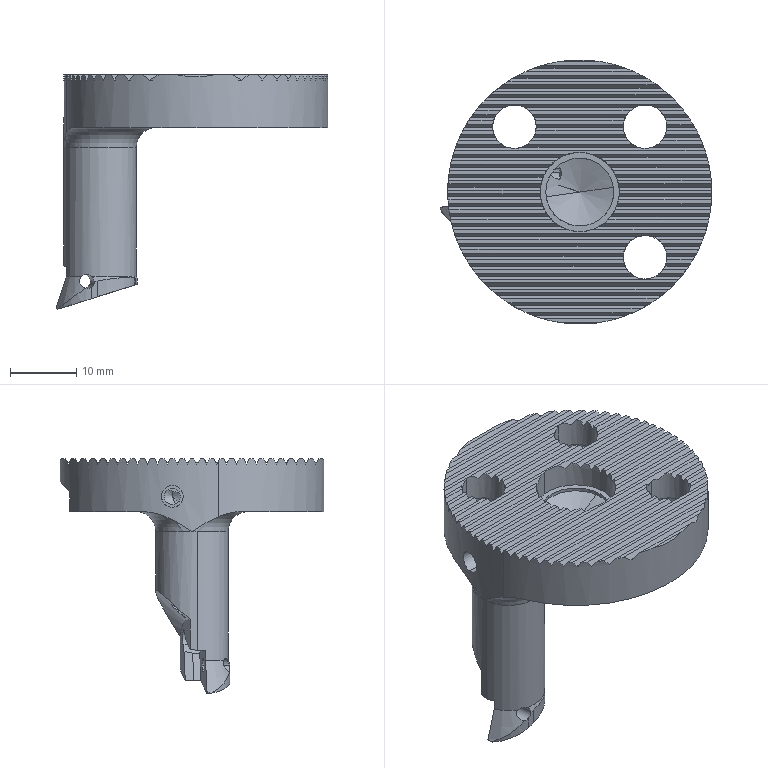Part | 1 solid | 203 faces | box 41.132 x 40 x 35.536 mm | volume 9670 mm3 | plane 160 | cylinder 34 | cone 7 | torus 2 | commonest cylinder face diameters 6.6 x6 10.5 x6 12 x3 2 x2 2.1 x2 2.5 x2